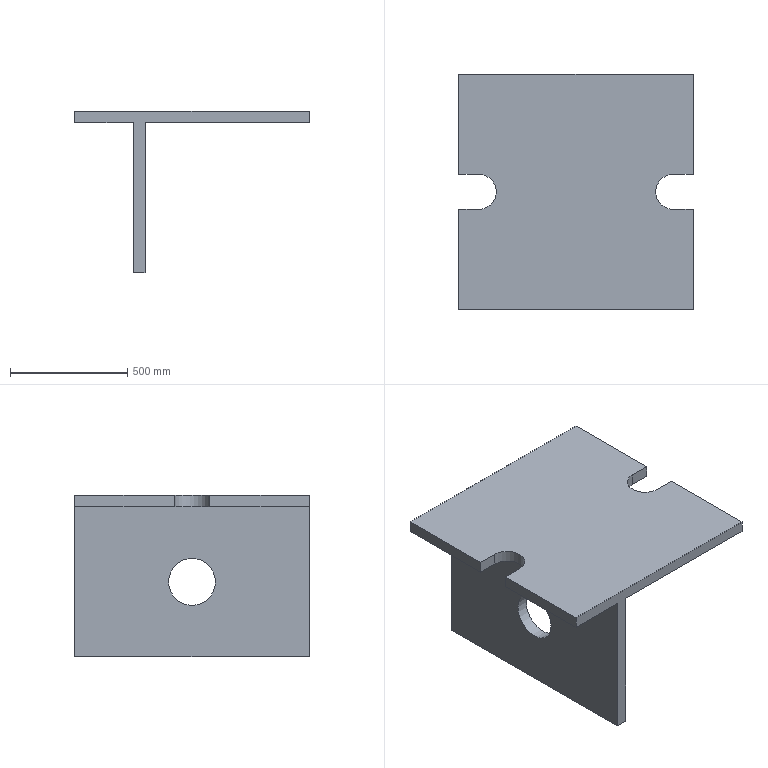Part | NX | features DATUM_CSYS 4, EXTRUDE 3, SKETCH 3, DATUM_PLANE 2, BLEND 1 | 1 solid | 19 faces | box 1000 x 1000 x 690 mm | volume 78270631 mm3 | plane 16 | cylinder 3 | commonest cylinder face diameters 150 x2 200 x1
STEP:
#1=CARTESIAN_POINT('',(415.,75.,0.));
#2=VERTEX_POINT('',#1);
#3=CARTESIAN_POINT('',(500.,75.,0.));
#4=VERTEX_POINT('',#3);
#5=CARTESIAN_POINT('',(340.,75.,0.));
#6=DIRECTION('',(1.,0.,0.));
#7=VECTOR('',#6,1000.);
#8=LINE('',#5,#7);
#9=EDGE_CURVE('',#2,#4,#8,.T.);
#10=ORIENTED_EDGE('',*,*,#9,.F.);
#11=CARTESIAN_POINT('',(415.,-75.,0.));
#12=VERTEX_POINT('',#11);
#13=CARTESIAN_POINT('',(415.,0.,0.));
#14=DIRECTION('',(0.,0.,1.));
#15=DIRECTION('',(1.,0.,0.));
#16=AXIS2_PLACEMENT_3D('',#13,#14,#15);
#17=CIRCLE('',#16,75.);
#18=EDGE_CURVE('',#2,#12,#17,.T.);
#19=ORIENTED_EDGE('',*,*,#18,.T.);
#20=CARTESIAN_POINT('',(500.,-75.,0.));
#21=VERTEX_POINT('',#20);
#22=CARTESIAN_POINT('',(560.,-75.,0.));
#23=DIRECTION('',(-1.,0.,0.));
#24=VECTOR('',#23,1000.);
#25=LINE('',#22,#24);
#26=EDGE_CURVE('',#21,#12,#25,.T.);
#27=ORIENTED_EDGE('',*,*,#26,.F.);
#28=CARTESIAN_POINT('',(500.,-500.,0.));
#29=VERTEX_POINT('',#28);
#30=CARTESIAN_POINT('',(500.,500.,0.));
#31=DIRECTION('',(0.,-1.,0.));
#32=VECTOR('',#31,1000.);
#33=LINE('',#30,#32);
#34=EDGE_CURVE('',#21,#29,#33,.T.);
#35=ORIENTED_EDGE('',*,*,#34,.T.);
#36=CARTESIAN_POINT('',(-200.,-500.,0.));
#37=VERTEX_POINT('',#36);
#38=CARTESIAN_POINT('',(500.,-500.,0.));
#39=DIRECTION('',(-1.,0.,0.));
#40=VECTOR('',#39,1000.);
#41=LINE('',#38,#40);
#42=EDGE_CURVE('',#29,#37,#41,.T.);
#43=ORIENTED_EDGE('',*,*,#42,.T.);
#44=CARTESIAN_POINT('',(-200.,500.,0.));
#45=VERTEX_POINT('',#44);
#46=CARTESIAN_POINT('',(-200.,500.,0.));
#47=DIRECTION('',(0.,-1.,0.));
#48=VECTOR('',#47,1000.);
#49=LINE('',#46,#48);
#50=EDGE_CURVE('',#45,#37,#49,.T.);
#51=ORIENTED_EDGE('',*,*,#50,.F.);
#52=CARTESIAN_POINT('',(500.,500.,0.));
#53=VERTEX_POINT('',#52);
#54=CARTESIAN_POINT('',(500.,500.,0.));
#55=DIRECTION('',(-1.,0.,0.));
#56=VECTOR('',#55,1000.);
#57=LINE('',#54,#56);
#58=EDGE_CURVE('',#53,#45,#57,.T.);
#59=ORIENTED_EDGE('',*,*,#58,.F.);
#60=CARTESIAN_POINT('',(500.,500.,0.));
#61=DIRECTION('',(0.,-1.,0.));
#62=VECTOR('',#61,1000.);
#63=LINE('',#60,#62);
#64=EDGE_CURVE('',#53,#4,#63,.T.);
#65=ORIENTED_EDGE('',*,*,#64,.T.);
#66=EDGE_LOOP('',(#10,#19,#27,#35,#43,#51,#59,#65));
#67=FACE_BOUND('',#66,.T.);
#68=CARTESIAN_POINT('',(500.,500.,0.));
#69=DIRECTION('',(0.,0.,1.));
#70=DIRECTION('',(1.,0.,0.));
#71=AXIS2_PLACEMENT_3D('',#68,#69,#70);
#72=PLANE('',#71);
#73=ADVANCED_FACE('',(#67),#72,.F.);
#74=CARTESIAN_POINT('',(500.,500.,50.));
#75=VERTEX_POINT('',#74);
#76=CARTESIAN_POINT('',(500.,75.,50.));
#77=VERTEX_POINT('',#76);
#78=CARTESIAN_POINT('',(500.,500.,50.));
#79=DIRECTION('',(0.,-1.,0.));
#80=VECTOR('',#79,1000.);
#81=LINE('',#78,#80);
#82=EDGE_CURVE('',#75,#77,#81,.T.);
#83=ORIENTED_EDGE('',*,*,#82,.T.);
#84=CARTESIAN_POINT('',(500.,75.,50.));
#85=DIRECTION('',(0.,0.,-1.));
#86=VECTOR('',#85,1000.);
#87=LINE('',#84,#86);
#88=EDGE_CURVE('',#77,#4,#87,.T.);
#89=ORIENTED_EDGE('',*,*,#88,.T.);
#90=ORIENTED_EDGE('',*,*,#64,.F.);
#91=CARTESIAN_POINT('',(500.,500.,50.));
#92=DIRECTION('',(0.,0.,-1.));
#93=VECTOR('',#92,1000.);
#94=LINE('',#91,#93);
#95=EDGE_CURVE('',#75,#53,#94,.T.);
#96=ORIENTED_EDGE('',*,*,#95,.F.);
#97=EDGE_LOOP('',(#83,#89,#90,#96));
#98=FACE_BOUND('',#97,.T.);
#99=CARTESIAN_POINT('',(500.,500.,50.));
#100=DIRECTION('',(-1.,0.,0.));
#101=DIRECTION('',(0.,0.,1.));
#102=AXIS2_PLACEMENT_3D('',#99,#100,#101);
#103=PLANE('',#102);
#104=ADVANCED_FACE('',(#98),#103,.F.);
#105=CARTESIAN_POINT('',(-500.,75.,0.));
#106=VERTEX_POINT('',#105);
#107=CARTESIAN_POINT('',(-415.,75.,0.));
#108=VERTEX_POINT('',#107);
#109=CARTESIAN_POINT('',(-560.,75.,0.));
#110=DIRECTION('',(1.,0.,0.));
#111=VECTOR('',#110,1000.);
#112=LINE('',#109,#111);
#113=EDGE_CURVE('',#106,#108,#112,.T.);
#114=ORIENTED_EDGE('',*,*,#113,.F.);
#115=CARTESIAN_POINT('',(-500.,500.,0.));
#116=VERTEX_POINT('',#115);
#117=CARTESIAN_POINT('',(-500.,500.,0.));
#118=DIRECTION('',(0.,-1.,0.));
#119=VECTOR('',#118,1000.);
#120=LINE('',#117,#119);
#121=EDGE_CURVE('',#116,#106,#120,.T.);
#122=ORIENTED_EDGE('',*,*,#121,.F.);
#123=CARTESIAN_POINT('',(-250.,500.,0.));
#124=VERTEX_POINT('',#123);
#125=CARTESIAN_POINT('',(-250.,500.,0.));
#126=DIRECTION('',(-1.,0.,0.));
#127=VECTOR('',#126,1000.);
#128=LINE('',#125,#127);
#129=EDGE_CURVE('',#124,#116,#128,.T.);
#130=ORIENTED_EDGE('',*,*,#129,.F.);
#131=CARTESIAN_POINT('',(-250.,-500.,0.));
#132=VERTEX_POINT('',#131);
#133=CARTESIAN_POINT('',(-250.,500.,0.));
#134=DIRECTION('',(0.,-1.,0.));
#135=VECTOR('',#134,1000.);
#136=LINE('',#133,#135);
#137=EDGE_CURVE('',#124,#132,#136,.T.);
#138=ORIENTED_EDGE('',*,*,#137,.T.);
#139=CARTESIAN_POINT('',(-500.,-500.,0.));
#140=VERTEX_POINT('',#139);
#141=CARTESIAN_POINT('',(-250.,-500.,0.));
#142=DIRECTION('',(-1.,0.,0.));
#143=VECTOR('',#142,1000.);
#144=LINE('',#141,#143);
#145=EDGE_CURVE('',#132,#140,#144,.T.);
#146=ORIENTED_EDGE('',*,*,#145,.T.);
#147=CARTESIAN_POINT('',(-500.,-75.,0.));
#148=VERTEX_POINT('',#147);
#149=CARTESIAN_POINT('',(-500.,500.,0.));
#150=DIRECTION('',(0.,-1.,0.));
#151=VECTOR('',#150,1000.);
#152=LINE('',#149,#151);
#153=EDGE_CURVE('',#148,#140,#152,.T.);
#154=ORIENTED_EDGE('',*,*,#153,.F.);
#155=CARTESIAN_POINT('',(-415.,-75.,0.));
#156=VERTEX_POINT('',#155);
#157=CARTESIAN_POINT('',(-340.,-75.,0.));
#158=DIRECTION('',(-1.,0.,0.));
#159=VECTOR('',#158,1000.);
#160=LINE('',#157,#159);
#161=EDGE_CURVE('',#156,#148,#160,.T.);
#162=ORIENTED_EDGE('',*,*,#161,.F.);
#163=CARTESIAN_POINT('',(-415.,0.,0.));
#164=DIRECTION('',(0.,0.,1.));
#165=DIRECTION('',(1.,0.,0.));
#166=AXIS2_PLACEMENT_3D('',#163,#164,#165);
#167=CIRCLE('',#166,75.);
#168=EDGE_CURVE('',#156,#108,#167,.T.);
#169=ORIENTED_EDGE('',*,*,#168,.T.);
#170=EDGE_LOOP('',(#114,#122,#130,#138,#146,#154,#162,#169));
#171=FACE_BOUND('',#170,.T.);
#172=CARTESIAN_POINT('',(-250.,500.,0.));
#173=DIRECTION('',(0.,0.,1.));
#174=DIRECTION('',(1.,0.,0.));
#175=AXIS2_PLACEMENT_3D('',#172,#173,#174);
#176=PLANE('',#175);
#177=ADVANCED_FACE('',(#171),#176,.F.);
#178=ORIENTED_EDGE('',*,*,#121,.T.);
#179=CARTESIAN_POINT('',(-500.,75.,50.));
#180=VERTEX_POINT('',#179);
#181=CARTESIAN_POINT('',(-500.,75.,0.));
#182=DIRECTION('',(0.,0.,1.));
#183=VECTOR('',#182,1000.);
#184=LINE('',#181,#183);
#185=EDGE_CURVE('',#106,#180,#184,.T.);
#186=ORIENTED_EDGE('',*,*,#185,.T.);
#187=CARTESIAN_POINT('',(-500.,500.,50.));
#188=VERTEX_POINT('',#187);
#189=CARTESIAN_POINT('',(-500.,500.,50.));
#190=DIRECTION('',(0.,-1.,0.));
#191=VECTOR('',#190,1000.);
#192=LINE('',#189,#191);
#193=EDGE_CURVE('',#188,#180,#192,.T.);
#194=ORIENTED_EDGE('',*,*,#193,.F.);
#195=CARTESIAN_POINT('',(-500.,500.,0.));
#196=DIRECTION('',(0.,0.,1.));
#197=VECTOR('',#196,1000.);
#198=LINE('',#195,#197);
#199=EDGE_CURVE('',#116,#188,#198,.T.);
#200=ORIENTED_EDGE('',*,*,#199,.F.);
#201=EDGE_LOOP('',(#178,#186,#194,#200));
#202=FACE_BOUND('',#201,.T.);
#203=CARTESIAN_POINT('',(-500.,500.,0.));
#204=DIRECTION('',(1.,0.,0.));
#205=DIRECTION('',(0.,0.,-1.));
#206=AXIS2_PLACEMENT_3D('',#203,#204,#205);
#207=PLANE('',#206);
#208=ADVANCED_FACE('',(#202),#207,.F.);
#209=CARTESIAN_POINT('',(-500.,-75.,50.));
#210=VERTEX_POINT('',#209);
#211=CARTESIAN_POINT('',(-500.,-500.,50.));
#212=VERTEX_POINT('',#211);
#213=CARTESIAN_POINT('',(-500.,500.,50.));
#214=DIRECTION('',(0.,-1.,0.));
#215=VECTOR('',#214,1000.);
#216=LINE('',#213,#215);
#217=EDGE_CURVE('',#210,#212,#216,.T.);
#218=ORIENTED_EDGE('',*,*,#217,.F.);
#219=CARTESIAN_POINT('',(-500.,-75.,0.));
#220=DIRECTION('',(0.,0.,-1.));
#221=VECTOR('',#220,1000.);
#222=LINE('',#219,#221);
#223=EDGE_CURVE('',#210,#148,#222,.T.);
#224=ORIENTED_EDGE('',*,*,#223,.T.);
#225=ORIENTED_EDGE('',*,*,#153,.T.);
#226=CARTESIAN_POINT('',(-500.,-500.,0.));
#227=DIRECTION('',(0.,0.,1.));
#228=VECTOR('',#227,1000.);
#229=LINE('',#226,#228);
#230=EDGE_CURVE('',#140,#212,#229,.T.);
#231=ORIENTED_EDGE('',*,*,#230,.T.);
#232=EDGE_LOOP('',(#218,#224,#225,#231));
#233=FACE_BOUND('',#232,.T.);
#234=CARTESIAN_POINT('',(-500.,500.,0.));
#235=DIRECTION('',(1.,0.,0.));
#236=DIRECTION('',(0.,0.,-1.));
#237=AXIS2_PLACEMENT_3D('',#234,#235,#236);
#238=PLANE('',#237);
#239=ADVANCED_FACE('',(#233),#238,.F.);
#240=CARTESIAN_POINT('',(500.,-75.,50.));
#241=VERTEX_POINT('',#240);
#242=CARTESIAN_POINT('',(500.,-500.,50.));
#243=VERTEX_POINT('',#242);
#244=CARTESIAN_POINT('',(500.,500.,50.));
#245=DIRECTION('',(0.,-1.,0.));
#246=VECTOR('',#245,1000.);
#247=LINE('',#244,#246);
#248=EDGE_CURVE('',#241,#243,#247,.T.);
#249=ORIENTED_EDGE('',*,*,#248,.F.);
#250=CARTESIAN_POINT('',(415.,-75.,50.));
#251=VERTEX_POINT('',#250);
#252=CARTESIAN_POINT('',(560.,-75.,50.));
#253=DIRECTION('',(-1.,0.,0.));
#254=VECTOR('',#253,1000.);
#255=LINE('',#252,#254);
#256=EDGE_CURVE('',#241,#251,#255,.T.);
#257=ORIENTED_EDGE('',*,*,#256,.T.);
#258=CARTESIAN_POINT('',(415.,75.,50.));
#259=VERTEX_POINT('',#258);
#260=CARTESIAN_POINT('',(415.,0.,50.));
#261=DIRECTION('',(0.,0.,-1.));
#262=DIRECTION('',(-1.,0.,0.));
#263=AXIS2_PLACEMENT_3D('',#260,#261,#262);
#264=CIRCLE('',#263,75.);
#265=EDGE_CURVE('',#251,#259,#264,.T.);
#266=ORIENTED_EDGE('',*,*,#265,.T.);
#267=CARTESIAN_POINT('',(340.,75.,50.));
#268=DIRECTION('',(1.,0.,0.));
#269=VECTOR('',#268,1000.);
#270=LINE('',#267,#269);
#271=EDGE_CURVE('',#259,#77,#270,.T.);
#272=ORIENTED_EDGE('',*,*,#271,.T.);
#273=ORIENTED_EDGE('',*,*,#82,.F.);
#274=CARTESIAN_POINT('',(-500.,500.,50.));
#275=DIRECTION('',(1.,0.,0.));
#276=VECTOR('',#275,1000.);
#277=LINE('',#274,#276);
#278=EDGE_CURVE('',#188,#75,#277,.T.);
#279=ORIENTED_EDGE('',*,*,#278,.F.);
#280=ORIENTED_EDGE('',*,*,#193,.T.);
#281=CARTESIAN_POINT('',(-415.,75.,50.));
#282=VERTEX_POINT('',#281);
#283=CARTESIAN_POINT('',(-560.,75.,50.));
#284=DIRECTION('',(1.,0.,0.));
#285=VECTOR('',#284,1000.);
#286=LINE('',#283,#285);
#287=EDGE_CURVE('',#180,#282,#286,.T.);
#288=ORIENTED_EDGE('',*,*,#287,.T.);
#289=CARTESIAN_POINT('',(-415.,-75.,50.));
#290=VERTEX_POINT('',#289);
#291=CARTESIAN_POINT('',(-415.,0.,50.));
#292=DIRECTION('',(0.,0.,-1.));
#293=DIRECTION('',(-1.,0.,0.));
#294=AXIS2_PLACEMENT_3D('',#291,#292,#293);
#295=CIRCLE('',#294,75.);
#296=EDGE_CURVE('',#282,#290,#295,.T.);
#297=ORIENTED_EDGE('',*,*,#296,.T.);
#298=CARTESIAN_POINT('',(-340.,-75.,50.));
#299=DIRECTION('',(-1.,0.,0.));
#300=VECTOR('',#299,1000.);
#301=LINE('',#298,#300);
#302=EDGE_CURVE('',#290,#210,#301,.T.);
#303=ORIENTED_EDGE('',*,*,#302,.T.);
#304=ORIENTED_EDGE('',*,*,#217,.T.);
#305=CARTESIAN_POINT('',(-500.,-500.,50.));
#306=DIRECTION('',(1.,0.,0.));
#307=VECTOR('',#306,1000.);
#308=LINE('',#305,#307);
#309=EDGE_CURVE('',#212,#243,#308,.T.);
#310=ORIENTED_EDGE('',*,*,#309,.T.);
#311=EDGE_LOOP('',(#249,#257,#266,#272,#273,#279,#280,#288,#297,#303,#304,#310));
#312=FACE_BOUND('',#311,.T.);
#313=CARTESIAN_POINT('',(-500.,500.,50.));
#314=DIRECTION('',(0.,0.,-1.));
#315=DIRECTION('',(-1.,0.,0.));
#316=AXIS2_PLACEMENT_3D('',#313,#314,#315);
#317=PLANE('',#316);
#318=ADVANCED_FACE('',(#312),#317,.F.);
#319=ORIENTED_EDGE('',*,*,#34,.F.);
#320=CARTESIAN_POINT('',(500.,-75.,50.));
#321=DIRECTION('',(0.,0.,1.));
#322=VECTOR('',#321,1000.);
#323=LINE('',#320,#322);
#324=EDGE_CURVE('',#21,#241,#323,.T.);
#325=ORIENTED_EDGE('',*,*,#324,.T.);
#326=ORIENTED_EDGE('',*,*,#248,.T.);
#327=CARTESIAN_POINT('',(500.,-500.,50.));
#328=DIRECTION('',(0.,0.,-1.));
#329=VECTOR('',#328,1000.);
#330=LINE('',#327,#329);
#331=EDGE_CURVE('',#243,#29,#330,.T.);
#332=ORIENTED_EDGE('',*,*,#331,.T.);
#333=EDGE_LOOP('',(#319,#325,#326,#332));
#334=FACE_BOUND('',#333,.T.);
#335=CARTESIAN_POINT('',(500.,500.,50.));
#336=DIRECTION('',(-1.,0.,0.));
#337=DIRECTION('',(0.,0.,1.));
#338=AXIS2_PLACEMENT_3D('',#335,#336,#337);
#339=PLANE('',#338);
#340=ADVANCED_FACE('',(#334),#339,.F.);
#341=CARTESIAN_POINT('',(-200.,-100.,-320.));
#342=VERTEX_POINT('',#341);
#343=CARTESIAN_POINT('',(-200.,0.,-320.));
#344=DIRECTION('',(1.,0.,0.));
#345=DIRECTION('',(0.,-1.,0.));
#346=AXIS2_PLACEMENT_3D('',#343,#344,#345);
#347=CIRCLE('',#346,100.);
#348=EDGE_CURVE('',#342,#342,#347,.T.);
#349=ORIENTED_EDGE('',*,*,#348,.F.);
#350=EDGE_LOOP('',(#349));
#351=FACE_BOUND('',#350,.T.);
#352=CARTESIAN_POINT('',(-200.,-500.,-640.));
#353=VERTEX_POINT('',#352);
#354=CARTESIAN_POINT('',(-200.,-500.,0.));
#355=DIRECTION('',(0.,0.,-1.));
#356=VECTOR('',#355,1000.);
#357=LINE('',#354,#356);
#358=EDGE_CURVE('',#37,#353,#357,.T.);
#359=ORIENTED_EDGE('',*,*,#358,.T.);
#360=CARTESIAN_POINT('',(-200.,500.,-640.));
#361=VERTEX_POINT('',#360);
#362=CARTESIAN_POINT('',(-200.,500.,-640.));
#363=DIRECTION('',(0.,-1.,0.));
#364=VECTOR('',#363,1000.);
#365=LINE('',#362,#364);
#366=EDGE_CURVE('',#361,#353,#365,.T.);
#367=ORIENTED_EDGE('',*,*,#366,.F.);
#368=CARTESIAN_POINT('',(-200.,500.,0.));
#369=DIRECTION('',(0.,0.,-1.));
#370=VECTOR('',#369,1000.);
#371=LINE('',#368,#370);
#372=EDGE_CURVE('',#45,#361,#371,.T.);
#373=ORIENTED_EDGE('',*,*,#372,.F.);
#374=ORIENTED_EDGE('',*,*,#50,.T.);
#375=EDGE_LOOP('',(#359,#367,#373,#374));
#376=FACE_BOUND('',#375,.T.);
#377=CARTESIAN_POINT('',(-200.,500.,0.));
#378=DIRECTION('',(-1.,0.,0.));
#379=DIRECTION('',(0.,0.,1.));
#380=AXIS2_PLACEMENT_3D('',#377,#378,#379);
#381=PLANE('',#380);
#382=ADVANCED_FACE('',(#351,#376),#381,.F.);
#383=CARTESIAN_POINT('',(-250.,-500.,-640.));
#384=VERTEX_POINT('',#383);
#385=CARTESIAN_POINT('',(-200.,-500.,-640.));
#386=DIRECTION('',(-1.,0.,0.));
#387=VECTOR('',#386,1000.);
#388=LINE('',#385,#387);
#389=EDGE_CURVE('',#353,#384,#388,.T.);
#390=ORIENTED_EDGE('',*,*,#389,.T.);
#391=CARTESIAN_POINT('',(-250.,500.,-640.));
#392=VERTEX_POINT('',#391);
#393=CARTESIAN_POINT('',(-250.,500.,-640.));
#394=DIRECTION('',(0.,-1.,0.));
#395=VECTOR('',#394,1000.);
#396=LINE('',#393,#395);
#397=EDGE_CURVE('',#392,#384,#396,.T.);
#398=ORIENTED_EDGE('',*,*,#397,.F.);
#399=CARTESIAN_POINT('',(-200.,500.,-640.));
#400=DIRECTION('',(-1.,0.,0.));
#401=VECTOR('',#400,1000.);
#402=LINE('',#399,#401);
#403=EDGE_CURVE('',#361,#392,#402,.T.);
#404=ORIENTED_EDGE('',*,*,#403,.F.);
#405=ORIENTED_EDGE('',*,*,#366,.T.);
#406=EDGE_LOOP('',(#390,#398,#404,#405));
#407=FACE_BOUND('',#406,.T.);
#408=CARTESIAN_POINT('',(-200.,500.,-640.));
#409=DIRECTION('',(0.,0.,1.));
#410=DIRECTION('',(1.,0.,0.));
#411=AXIS2_PLACEMENT_3D('',#408,#409,#410);
#412=PLANE('',#411);
#413=ADVANCED_FACE('',(#407),#412,.F.);
#414=CARTESIAN_POINT('',(-250.,-100.,-320.));
#415=VERTEX_POINT('',#414);
#416=CARTESIAN_POINT('',(-250.,0.,-320.));
#417=DIRECTION('',(1.,0.,0.));
#418=DIRECTION('',(0.,-1.,0.));
#419=AXIS2_PLACEMENT_3D('',#416,#417,#418);
#420=CIRCLE('',#419,100.);
#421=EDGE_CURVE('',#415,#415,#420,.T.);
#422=ORIENTED_EDGE('',*,*,#421,.T.);
#423=EDGE_LOOP('',(#422));
#424=FACE_BOUND('',#423,.T.);
#425=CARTESIAN_POINT('',(-250.,-500.,-640.));
#426=DIRECTION('',(0.,0.,1.));
#427=VECTOR('',#426,1000.);
#428=LINE('',#425,#427);
#429=EDGE_CURVE('',#384,#132,#428,.T.);
#430=ORIENTED_EDGE('',*,*,#429,.T.);
#431=ORIENTED_EDGE('',*,*,#137,.F.);
#432=CARTESIAN_POINT('',(-250.,500.,-640.));
#433=DIRECTION('',(0.,0.,1.));
#434=VECTOR('',#433,1000.);
#435=LINE('',#432,#434);
#436=EDGE_CURVE('',#392,#124,#435,.T.);
#437=ORIENTED_EDGE('',*,*,#436,.F.);
#438=ORIENTED_EDGE('',*,*,#397,.T.);
#439=EDGE_LOOP('',(#430,#431,#437,#438));
#440=FACE_BOUND('',#439,.T.);
#441=CARTESIAN_POINT('',(-250.,500.,-640.));
#442=DIRECTION('',(1.,0.,0.));
#443=DIRECTION('',(0.,0.,-1.));
#444=AXIS2_PLACEMENT_3D('',#441,#442,#443);
#445=PLANE('',#444);
#446=ADVANCED_FACE('',(#424,#440),#445,.F.);
#447=ORIENTED_EDGE('',*,*,#199,.T.);
#448=ORIENTED_EDGE('',*,*,#278,.T.);
#449=ORIENTED_EDGE('',*,*,#95,.T.);
#450=ORIENTED_EDGE('',*,*,#58,.T.);
#451=ORIENTED_EDGE('',*,*,#372,.T.);
#452=ORIENTED_EDGE('',*,*,#403,.T.);
#453=ORIENTED_EDGE('',*,*,#436,.T.);
#454=ORIENTED_EDGE('',*,*,#129,.T.);
#455=EDGE_LOOP('',(#447,#448,#449,#450,#451,#452,#453,#454));
#456=FACE_BOUND('',#455,.T.);
#457=CARTESIAN_POINT('',(0.,500.,0.));
#458=DIRECTION('',(0.,1.,0.));
#459=DIRECTION('',(0.,0.,1.));
#460=AXIS2_PLACEMENT_3D('',#457,#458,#459);
#461=PLANE('',#460);
#462=ADVANCED_FACE('',(#456),#461,.T.);
#463=ORIENTED_EDGE('',*,*,#230,.F.);
#464=ORIENTED_EDGE('',*,*,#145,.F.);
#465=ORIENTED_EDGE('',*,*,#429,.F.);
#466=ORIENTED_EDGE('',*,*,#389,.F.);
#467=ORIENTED_EDGE('',*,*,#358,.F.);
#468=ORIENTED_EDGE('',*,*,#42,.F.);
#469=ORIENTED_EDGE('',*,*,#331,.F.);
#470=ORIENTED_EDGE('',*,*,#309,.F.);
#471=EDGE_LOOP('',(#463,#464,#465,#466,#467,#468,#469,#470));
#472=FACE_BOUND('',#471,.T.);
#473=CARTESIAN_POINT('',(0.,-500.,0.));
#474=DIRECTION('',(0.,1.,0.));
#475=DIRECTION('',(0.,0.,1.));
#476=AXIS2_PLACEMENT_3D('',#473,#474,#475);
#477=PLANE('',#476);
#478=ADVANCED_FACE('',(#472),#477,.F.);
#479=ORIENTED_EDGE('',*,*,#113,.T.);
#480=CARTESIAN_POINT('',(-415.,75.,50.));
#481=DIRECTION('',(0.,0.,1.));
#482=VECTOR('',#481,1000.);
#483=LINE('',#480,#482);
#484=EDGE_CURVE('',#108,#282,#483,.T.);
#485=ORIENTED_EDGE('',*,*,#484,.T.);
#486=ORIENTED_EDGE('',*,*,#287,.F.);
#487=ORIENTED_EDGE('',*,*,#185,.F.);
#488=EDGE_LOOP('',(#479,#485,#486,#487));
#489=FACE_BOUND('',#488,.T.);
#490=CARTESIAN_POINT('',(-560.,75.,50.));
#491=DIRECTION('',(0.,1.,0.));
#492=DIRECTION('',(0.,0.,1.));
#493=AXIS2_PLACEMENT_3D('',#490,#491,#492);
#494=PLANE('',#493);
#495=ADVANCED_FACE('',(#489),#494,.F.);
#496=ORIENTED_EDGE('',*,*,#302,.F.);
#497=CARTESIAN_POINT('',(-415.,-75.,0.));
#498=DIRECTION('',(0.,0.,1.));
#499=VECTOR('',#498,1000.);
#500=LINE('',#497,#499);
#501=EDGE_CURVE('',#290,#156,#500,.F.);
#502=ORIENTED_EDGE('',*,*,#501,.T.);
#503=ORIENTED_EDGE('',*,*,#161,.T.);
#504=ORIENTED_EDGE('',*,*,#223,.F.);
#505=EDGE_LOOP('',(#496,#502,#503,#504));
#506=FACE_BOUND('',#505,.T.);
#507=CARTESIAN_POINT('',(-340.,-75.,50.));
#508=DIRECTION('',(0.,-1.,0.));
#509=DIRECTION('',(0.,0.,-1.));
#510=AXIS2_PLACEMENT_3D('',#507,#508,#509);
#511=PLANE('',#510);
#512=ADVANCED_FACE('',(#506),#511,.F.);
#513=ORIENTED_EDGE('',*,*,#271,.F.);
#514=CARTESIAN_POINT('',(415.,75.,0.));
#515=DIRECTION('',(0.,0.,1.));
#516=VECTOR('',#515,1000.);
#517=LINE('',#514,#516);
#518=EDGE_CURVE('',#259,#2,#517,.F.);
#519=ORIENTED_EDGE('',*,*,#518,.T.);
#520=ORIENTED_EDGE('',*,*,#9,.T.);
#521=ORIENTED_EDGE('',*,*,#88,.F.);
#522=EDGE_LOOP('',(#513,#519,#520,#521));
#523=FACE_BOUND('',#522,.T.);
#524=CARTESIAN_POINT('',(340.,75.,50.));
#525=DIRECTION('',(0.,1.,0.));
#526=DIRECTION('',(0.,0.,1.));
#527=AXIS2_PLACEMENT_3D('',#524,#525,#526);
#528=PLANE('',#527);
#529=ADVANCED_FACE('',(#523),#528,.F.);
#530=ORIENTED_EDGE('',*,*,#26,.T.);
#531=CARTESIAN_POINT('',(415.,-75.,50.));
#532=DIRECTION('',(0.,0.,1.));
#533=VECTOR('',#532,1000.);
#534=LINE('',#531,#533);
#535=EDGE_CURVE('',#12,#251,#534,.T.);
#536=ORIENTED_EDGE('',*,*,#535,.T.);
#537=ORIENTED_EDGE('',*,*,#256,.F.);
#538=ORIENTED_EDGE('',*,*,#324,.F.);
#539=EDGE_LOOP('',(#530,#536,#537,#538));
#540=FACE_BOUND('',#539,.T.);
#541=CARTESIAN_POINT('',(560.,-75.,50.));
#542=DIRECTION('',(0.,-1.,0.));
#543=DIRECTION('',(0.,0.,-1.));
#544=AXIS2_PLACEMENT_3D('',#541,#542,#543);
#545=PLANE('',#544);
#546=ADVANCED_FACE('',(#540),#545,.F.);
#547=ORIENTED_EDGE('',*,*,#518,.F.);
#548=ORIENTED_EDGE('',*,*,#265,.F.);
#549=ORIENTED_EDGE('',*,*,#535,.F.);
#550=ORIENTED_EDGE('',*,*,#18,.F.);
#551=EDGE_LOOP('',(#547,#548,#549,#550));
#552=FACE_BOUND('',#551,.T.);
#553=CARTESIAN_POINT('',(415.,0.,50.));
#554=DIRECTION('',(0.,0.,-1.));
#555=DIRECTION('',(-1.,0.,0.));
#556=AXIS2_PLACEMENT_3D('',#553,#554,#555);
#557=CYLINDRICAL_SURFACE('',#556,75.);
#558=ADVANCED_FACE('',(#552),#557,.F.);
#559=ORIENTED_EDGE('',*,*,#501,.F.);
#560=ORIENTED_EDGE('',*,*,#296,.F.);
#561=ORIENTED_EDGE('',*,*,#484,.F.);
#562=ORIENTED_EDGE('',*,*,#168,.F.);
#563=EDGE_LOOP('',(#559,#560,#561,#562));
#564=FACE_BOUND('',#563,.T.);
#565=CARTESIAN_POINT('',(-415.,0.,50.));
#566=DIRECTION('',(0.,0.,-1.));
#567=DIRECTION('',(-1.,0.,0.));
#568=AXIS2_PLACEMENT_3D('',#565,#566,#567);
#569=CYLINDRICAL_SURFACE('',#568,75.);
#570=ADVANCED_FACE('',(#564),#569,.F.);
#571=ORIENTED_EDGE('',*,*,#421,.F.);
#572=EDGE_LOOP('',(#571));
#573=FACE_BOUND('',#572,.T.);
#574=ORIENTED_EDGE('',*,*,#348,.T.);
#575=EDGE_LOOP('',(#574));
#576=FACE_BOUND('',#575,.T.);
#577=CARTESIAN_POINT('',(-250.,0.,-320.));
#578=DIRECTION('',(1.,0.,0.));
#579=DIRECTION('',(0.,0.,-1.));
#580=AXIS2_PLACEMENT_3D('',#577,#578,#579);
#581=CYLINDRICAL_SURFACE('',#580,100.);
#582=ADVANCED_FACE('',(#573,#576),#581,.F.);
#583=CLOSED_SHELL('',(#73,#104,#177,#208,#239,#318,#340,#382,#413,#446,#462,#478,#495,#512,#529,#546,#558,#570,#582));
#584=MANIFOLD_SOLID_BREP('',#583);
#585=(LENGTH_UNIT()NAMED_UNIT(*)SI_UNIT(.MILLI.,.METRE.));
#586=UNCERTAINTY_MEASURE_WITH_UNIT(LENGTH_MEASURE(0.00001),#585,'','');
#587=(NAMED_UNIT(*)PLANE_ANGLE_UNIT()SI_UNIT($,.RADIAN.));
#588=(NAMED_UNIT(*)SI_UNIT($,.STERADIAN.)SOLID_ANGLE_UNIT());
#589=(GEOMETRIC_REPRESENTATION_CONTEXT(3)GLOBAL_UNCERTAINTY_ASSIGNED_CONTEXT((#586))GLOBAL_UNIT_ASSIGNED_CONTEXT((#585,#587,#588))REPRESENTATION_CONTEXT('',''));
#590=ADVANCED_BREP_SHAPE_REPRESENTATION('',(#584),#589);